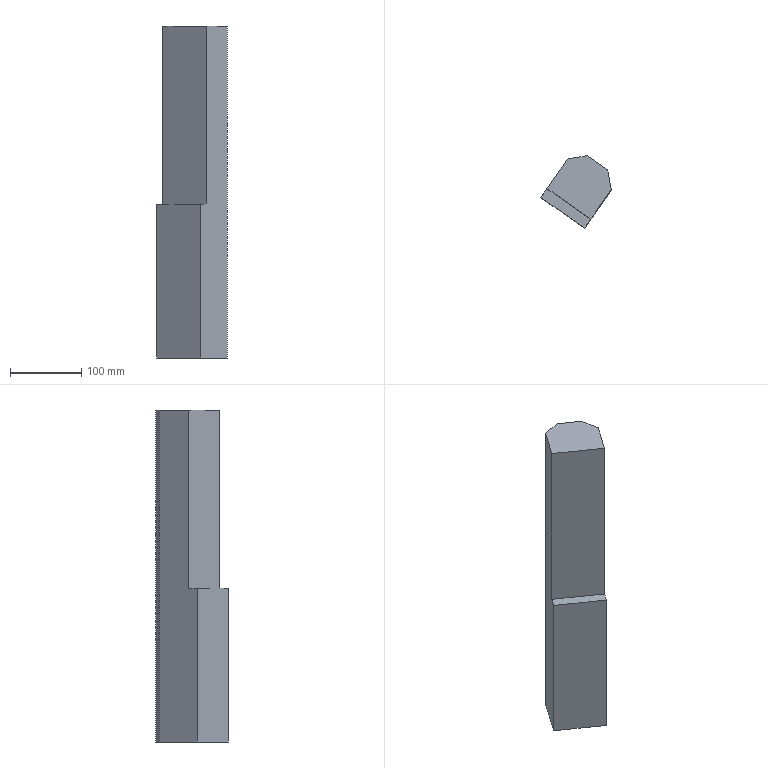Part | NX | features solid 2 | 1 solid | 20 faces | box 98.719 x 101.175 x 465 mm | volume 2453936 mm3 | plane 12 | cylinder 5 | cone 3 | commonest cylinder face diameters 16 x5
STEP:
#1=CARTESIAN_POINT('',(345.382,545.56,-124.062));
#2=VERTEX_POINT('',#1);
#3=CARTESIAN_POINT('',(374.061,586.518,-124.062));
#4=VERTEX_POINT('',#3);
#5=CARTESIAN_POINT('',(345.382,545.56,-124.062));
#6=DIRECTION('',(-0.5736,-0.8192,0.));
#7=VECTOR('',#6,1000.);
#8=LINE('',#5,#7);
#9=EDGE_CURVE('',#2,#4,#8,.F.);
#10=ORIENTED_EDGE('',*,*,#9,.T.);
#11=CARTESIAN_POINT('',(369.15,614.373,-124.062));
#12=VERTEX_POINT('',#11);
#13=CARTESIAN_POINT('',(374.061,586.518,-124.062));
#14=DIRECTION('',(-0.1736,0.9848,0.));
#15=VECTOR('',#14,1000.);
#16=LINE('',#13,#15);
#17=EDGE_CURVE('',#4,#12,#16,.T.);
#18=ORIENTED_EDGE('',*,*,#17,.T.);
#19=CARTESIAN_POINT('',(340.479,634.448,-124.062));
#20=VERTEX_POINT('',#19);
#21=CARTESIAN_POINT('',(324.096,645.919,-124.062));
#22=DIRECTION('',(-0.8192,0.5736,0.));
#23=VECTOR('',#22,1000.);
#24=LINE('',#21,#23);
#25=EDGE_CURVE('',#12,#20,#24,.T.);
#26=ORIENTED_EDGE('',*,*,#25,.T.);
#27=CARTESIAN_POINT('',(312.625,629.536,-124.062));
#28=VERTEX_POINT('',#27);
#29=CARTESIAN_POINT('',(312.625,629.536,-124.062));
#30=DIRECTION('',(-0.9848,-0.1736,0.));
#31=VECTOR('',#30,1000.);
#32=LINE('',#29,#31);
#33=EDGE_CURVE('',#20,#28,#32,.T.);
#34=ORIENTED_EDGE('',*,*,#33,.T.);
#35=CARTESIAN_POINT('',(283.946,588.579,-124.062));
#36=VERTEX_POINT('',#35);
#37=CARTESIAN_POINT('',(283.946,588.579,-124.062));
#38=DIRECTION('',(0.5736,0.8192,0.));
#39=VECTOR('',#38,1000.);
#40=LINE('',#37,#39);
#41=EDGE_CURVE('',#36,#28,#40,.T.);
#42=ORIENTED_EDGE('',*,*,#41,.F.);
#43=CARTESIAN_POINT('',(283.946,588.579,-124.062));
#44=DIRECTION('',(0.8192,-0.5736,0.));
#45=VECTOR('',#44,1000.);
#46=LINE('',#43,#45);
#47=EDGE_CURVE('',#36,#2,#46,.T.);
#48=ORIENTED_EDGE('',*,*,#47,.T.);
#49=EDGE_LOOP('',(#10,#18,#26,#34,#42,#48));
#50=FACE_BOUND('',#49,.T.);
#51=CARTESIAN_POINT('',(283.946,588.579,-124.062));
#52=DIRECTION('',(0.,0.,-1.));
#53=DIRECTION('',(0.5736,0.8192,0.));
#54=AXIS2_PLACEMENT_3D('',#51,#52,#53);
#55=PLANE('',#54);
#56=ADVANCED_FACE('',(#50),#55,.F.);
#57=CARTESIAN_POINT('',(345.382,545.56,-374.062));
#58=VERTEX_POINT('',#57);
#59=CARTESIAN_POINT('',(345.382,545.56,-401.082));
#60=DIRECTION('',(0.,0.,-1.));
#61=VECTOR('',#60,1000.);
#62=LINE('',#59,#61);
#63=EDGE_CURVE('',#2,#58,#62,.T.);
#64=ORIENTED_EDGE('',*,*,#63,.F.);
#65=ORIENTED_EDGE('',*,*,#47,.F.);
#66=CARTESIAN_POINT('',(283.946,588.579,-374.062));
#67=VERTEX_POINT('',#66);
#68=CARTESIAN_POINT('',(283.946,588.579,-401.082));
#69=DIRECTION('',(0.,0.,-1.));
#70=VECTOR('',#69,1000.);
#71=LINE('',#68,#70);
#72=EDGE_CURVE('',#36,#67,#71,.T.);
#73=ORIENTED_EDGE('',*,*,#72,.T.);
#74=CARTESIAN_POINT('',(337.191,551.296,-374.062));
#75=DIRECTION('',(-0.8192,0.5736,0.));
#76=VECTOR('',#75,1000.);
#77=LINE('',#74,#76);
#78=EDGE_CURVE('',#58,#67,#77,.T.);
#79=ORIENTED_EDGE('',*,*,#78,.F.);
#80=EDGE_LOOP('',(#64,#65,#73,#79));
#81=FACE_BOUND('',#80,.T.);
#82=CARTESIAN_POINT('',(283.946,588.579,-401.082));
#83=DIRECTION('',(0.5736,0.8192,0.));
#84=DIRECTION('',(0.8192,-0.5736,0.));
#85=AXIS2_PLACEMENT_3D('',#82,#83,#84);
#86=PLANE('',#85);
#87=ADVANCED_FACE('',(#81),#86,.F.);
#88=CARTESIAN_POINT('',(336.779,533.273,-374.062));
#89=VERTEX_POINT('',#88);
#90=CARTESIAN_POINT('',(336.779,533.273,-589.062));
#91=VERTEX_POINT('',#90);
#92=CARTESIAN_POINT('',(336.779,533.273,-461.082));
#93=DIRECTION('',(0.,0.,1.));
#94=VECTOR('',#93,1000.);
#95=LINE('',#92,#94);
#96=EDGE_CURVE('',#89,#91,#95,.F.);
#97=ORIENTED_EDGE('',*,*,#96,.F.);
#98=CARTESIAN_POINT('',(275.342,576.291,-374.062));
#99=VERTEX_POINT('',#98);
#100=CARTESIAN_POINT('',(328.587,539.009,-374.062));
#101=DIRECTION('',(-0.8192,0.5736,0.));
#102=VECTOR('',#101,1000.);
#103=LINE('',#100,#102);
#104=EDGE_CURVE('',#89,#99,#103,.T.);
#105=ORIENTED_EDGE('',*,*,#104,.T.);
#106=CARTESIAN_POINT('',(275.342,576.291,-589.062));
#107=VERTEX_POINT('',#106);
#108=CARTESIAN_POINT('',(275.342,576.291,-401.082));
#109=DIRECTION('',(0.,0.,-1.));
#110=VECTOR('',#109,1000.);
#111=LINE('',#108,#110);
#112=EDGE_CURVE('',#99,#107,#111,.T.);
#113=ORIENTED_EDGE('',*,*,#112,.T.);
#114=CARTESIAN_POINT('',(275.26,576.349,-589.062));
#115=DIRECTION('',(0.8192,-0.5736,0.));
#116=VECTOR('',#115,1000.);
#117=LINE('',#114,#116);
#118=EDGE_CURVE('',#91,#107,#117,.F.);
#119=ORIENTED_EDGE('',*,*,#118,.F.);
#120=EDGE_LOOP('',(#97,#105,#113,#119));
#121=FACE_BOUND('',#120,.T.);
#122=CARTESIAN_POINT('',(328.587,539.009,-461.082));
#123=DIRECTION('',(-0.5736,-0.8192,0.));
#124=DIRECTION('',(-0.8192,0.5736,0.));
#125=AXIS2_PLACEMENT_3D('',#122,#123,#124);
#126=PLANE('',#125);
#127=ADVANCED_FACE('',(#121),#126,.T.);
#128=CARTESIAN_POINT('',(341.074,585.702,-589.062));
#129=VERTEX_POINT('',#128);
#130=CARTESIAN_POINT('',(349.074,585.702,-589.062));
#131=DIRECTION('',(0.,0.,-1.));
#132=DIRECTION('',(-1.,0.,0.));
#133=AXIS2_PLACEMENT_3D('',#130,#131,#132);
#134=CIRCLE('',#133,8.);
#135=EDGE_CURVE('',#129,#129,#134,.F.);
#136=ORIENTED_EDGE('',*,*,#135,.T.);
#137=EDGE_LOOP('',(#136));
#138=FACE_BOUND('',#137,.T.);
#139=CARTESIAN_POINT('',(309.536,601.682,-589.062));
#140=VERTEX_POINT('',#139);
#141=CARTESIAN_POINT('',(317.536,601.682,-589.062));
#142=DIRECTION('',(0.,0.,-1.));
#143=DIRECTION('',(-1.,0.,0.));
#144=AXIS2_PLACEMENT_3D('',#141,#142,#143);
#145=CIRCLE('',#144,8.);
#146=EDGE_CURVE('',#140,#140,#145,.F.);
#147=ORIENTED_EDGE('',*,*,#146,.T.);
#148=EDGE_LOOP('',(#147));
#149=FACE_BOUND('',#148,.T.);
#150=CARTESIAN_POINT('',(349.295,609.461,-589.062));
#151=VERTEX_POINT('',#150);
#152=CARTESIAN_POINT('',(341.295,609.461,-589.062));
#153=DIRECTION('',(0.,0.,1.));
#154=DIRECTION('',(1.,0.,0.));
#155=AXIS2_PLACEMENT_3D('',#152,#153,#154);
#156=CIRCLE('',#155,8.);
#157=EDGE_CURVE('',#151,#151,#156,.T.);
#158=ORIENTED_EDGE('',*,*,#157,.T.);
#159=EDGE_LOOP('',(#158));
#160=FACE_BOUND('',#159,.T.);
#161=CARTESIAN_POINT('',(311.197,581.203,-589.062));
#162=VERTEX_POINT('',#161);
#163=CARTESIAN_POINT('',(303.197,581.203,-589.062));
#164=DIRECTION('',(0.,0.,1.));
#165=DIRECTION('',(1.,0.,0.));
#166=AXIS2_PLACEMENT_3D('',#163,#164,#165);
#167=CIRCLE('',#166,8.);
#168=EDGE_CURVE('',#162,#162,#167,.T.);
#169=ORIENTED_EDGE('',*,*,#168,.T.);
#170=EDGE_LOOP('',(#169));
#171=FACE_BOUND('',#170,.T.);
#172=CARTESIAN_POINT('',(339.867,561.128,-589.062));
#173=VERTEX_POINT('',#172);
#174=CARTESIAN_POINT('',(331.867,561.128,-589.062));
#175=DIRECTION('',(0.,0.,1.));
#176=DIRECTION('',(1.,0.,0.));
#177=AXIS2_PLACEMENT_3D('',#174,#175,#176);
#178=CIRCLE('',#177,8.);
#179=EDGE_CURVE('',#173,#173,#178,.T.);
#180=ORIENTED_EDGE('',*,*,#179,.T.);
#181=EDGE_LOOP('',(#180));
#182=FACE_BOUND('',#181,.T.);
#183=CARTESIAN_POINT('',(369.15,614.373,-589.062));
#184=VERTEX_POINT('',#183);
#185=CARTESIAN_POINT('',(340.479,634.448,-589.062));
#186=VERTEX_POINT('',#185);
#187=CARTESIAN_POINT('',(-187.66,1004.255,-589.062));
#188=DIRECTION('',(0.8192,-0.5736,0.));
#189=VECTOR('',#188,1000.);
#190=LINE('',#187,#189);
#191=EDGE_CURVE('',#184,#186,#190,.F.);
#192=ORIENTED_EDGE('',*,*,#191,.F.);
#193=CARTESIAN_POINT('',(374.061,586.518,-589.062));
#194=VERTEX_POINT('',#193);
#195=CARTESIAN_POINT('',(374.061,586.518,-589.062));
#196=DIRECTION('',(-0.1736,0.9848,0.));
#197=VECTOR('',#196,1000.);
#198=LINE('',#195,#197);
#199=EDGE_CURVE('',#184,#194,#198,.F.);
#200=ORIENTED_EDGE('',*,*,#199,.T.);
#201=CARTESIAN_POINT('',(256.478,418.592,-589.062));
#202=DIRECTION('',(0.5736,0.8192,0.));
#203=VECTOR('',#202,1000.);
#204=LINE('',#201,#203);
#205=EDGE_CURVE('',#91,#194,#204,.T.);
#206=ORIENTED_EDGE('',*,*,#205,.F.);
#207=ORIENTED_EDGE('',*,*,#118,.T.);
#208=CARTESIAN_POINT('',(312.625,629.536,-589.062));
#209=VERTEX_POINT('',#208);
#210=CARTESIAN_POINT('',(344.171,674.59,-589.062));
#211=DIRECTION('',(-0.5736,-0.8192,0.));
#212=VECTOR('',#211,1000.);
#213=LINE('',#210,#212);
#214=EDGE_CURVE('',#107,#209,#213,.F.);
#215=ORIENTED_EDGE('',*,*,#214,.T.);
#216=CARTESIAN_POINT('',(312.625,629.536,-589.062));
#217=DIRECTION('',(-0.9848,-0.1736,0.));
#218=VECTOR('',#217,1000.);
#219=LINE('',#216,#218);
#220=EDGE_CURVE('',#209,#186,#219,.F.);
#221=ORIENTED_EDGE('',*,*,#220,.T.);
#222=EDGE_LOOP('',(#192,#200,#206,#207,#215,#221));
#223=FACE_BOUND('',#222,.T.);
#224=CARTESIAN_POINT('',(344.089,674.647,-589.062));
#225=DIRECTION('',(0.,0.,-1.));
#226=DIRECTION('',(-0.5736,-0.8192,0.));
#227=AXIS2_PLACEMENT_3D('',#224,#225,#226);
#228=PLANE('',#227);
#229=ADVANCED_FACE('',(#138,#149,#160,#171,#182,#223),#228,.T.);
#230=ORIENTED_EDGE('',*,*,#41,.T.);
#231=CARTESIAN_POINT('',(312.625,629.536,-589.062));
#232=DIRECTION('',(0.,0.,-1.));
#233=VECTOR('',#232,1000.);
#234=LINE('',#231,#233);
#235=EDGE_CURVE('',#28,#209,#234,.T.);
#236=ORIENTED_EDGE('',*,*,#235,.T.);
#237=ORIENTED_EDGE('',*,*,#214,.F.);
#238=ORIENTED_EDGE('',*,*,#112,.F.);
#239=CARTESIAN_POINT('',(283.946,588.579,-374.062));
#240=DIRECTION('',(0.5736,0.8192,0.));
#241=VECTOR('',#240,1000.);
#242=LINE('',#239,#241);
#243=EDGE_CURVE('',#99,#67,#242,.T.);
#244=ORIENTED_EDGE('',*,*,#243,.T.);
#245=ORIENTED_EDGE('',*,*,#72,.F.);
#246=EDGE_LOOP('',(#230,#236,#237,#238,#244,#245));
#247=FACE_BOUND('',#246,.T.);
#248=CARTESIAN_POINT('',(283.946,588.579,-151.082));
#249=DIRECTION('',(-0.8192,0.5736,0.));
#250=DIRECTION('',(0.5736,0.8192,0.));
#251=AXIS2_PLACEMENT_3D('',#248,#249,#250);
#252=PLANE('',#251);
#253=ADVANCED_FACE('',(#247),#252,.T.);
#254=ORIENTED_EDGE('',*,*,#25,.F.);
#255=CARTESIAN_POINT('',(369.15,614.373,-192.696));
#256=DIRECTION('',(0.,0.,-1.));
#257=VECTOR('',#256,1000.);
#258=LINE('',#255,#257);
#259=EDGE_CURVE('',#12,#184,#258,.T.);
#260=ORIENTED_EDGE('',*,*,#259,.T.);
#261=ORIENTED_EDGE('',*,*,#191,.T.);
#262=CARTESIAN_POINT('',(340.479,634.448,-124.062));
#263=DIRECTION('',(0.,0.,1.));
#264=VECTOR('',#263,1000.);
#265=LINE('',#262,#264);
#266=EDGE_CURVE('',#186,#20,#265,.T.);
#267=ORIENTED_EDGE('',*,*,#266,.T.);
#268=EDGE_LOOP('',(#254,#260,#261,#267));
#269=FACE_BOUND('',#268,.T.);
#270=CARTESIAN_POINT('',(-187.66,1004.255,-192.696));
#271=DIRECTION('',(-0.5736,-0.8192,0.));
#272=DIRECTION('',(-0.8192,0.5736,0.));
#273=AXIS2_PLACEMENT_3D('',#270,#271,#272);
#274=PLANE('',#273);
#275=ADVANCED_FACE('',(#269),#274,.F.);
#276=CARTESIAN_POINT('',(345.382,545.56,-374.062));
#277=DIRECTION('',(0.5736,0.8192,0.));
#278=VECTOR('',#277,1000.);
#279=LINE('',#276,#278);
#280=EDGE_CURVE('',#89,#58,#279,.T.);
#281=ORIENTED_EDGE('',*,*,#280,.T.);
#282=ORIENTED_EDGE('',*,*,#78,.T.);
#283=ORIENTED_EDGE('',*,*,#243,.F.);
#284=ORIENTED_EDGE('',*,*,#104,.F.);
#285=EDGE_LOOP('',(#281,#282,#283,#284));
#286=FACE_BOUND('',#285,.T.);
#287=CARTESIAN_POINT('',(337.191,551.296,-374.062));
#288=DIRECTION('',(0.,0.,1.));
#289=DIRECTION('',(-0.5736,-0.8192,0.));
#290=AXIS2_PLACEMENT_3D('',#287,#288,#289);
#291=PLANE('',#290);
#292=ADVANCED_FACE('',(#286),#291,.T.);
#293=ORIENTED_EDGE('',*,*,#205,.T.);
#294=CARTESIAN_POINT('',(374.061,586.518,-400.));
#295=DIRECTION('',(0.,0.,-1.));
#296=VECTOR('',#295,1000.);
#297=LINE('',#294,#296);
#298=EDGE_CURVE('',#194,#4,#297,.F.);
#299=ORIENTED_EDGE('',*,*,#298,.T.);
#300=ORIENTED_EDGE('',*,*,#9,.F.);
#301=ORIENTED_EDGE('',*,*,#63,.T.);
#302=ORIENTED_EDGE('',*,*,#280,.F.);
#303=ORIENTED_EDGE('',*,*,#96,.T.);
#304=EDGE_LOOP('',(#293,#299,#300,#301,#302,#303));
#305=FACE_BOUND('',#304,.T.);
#306=CARTESIAN_POINT('',(256.478,418.592,-400.));
#307=DIRECTION('',(0.8192,-0.5736,0.));
#308=DIRECTION('',(0.,0.,1.));
#309=AXIS2_PLACEMENT_3D('',#306,#307,#308);
#310=PLANE('',#309);
#311=ADVANCED_FACE('',(#305),#310,.T.);
#312=ORIENTED_EDGE('',*,*,#33,.F.);
#313=ORIENTED_EDGE('',*,*,#266,.F.);
#314=ORIENTED_EDGE('',*,*,#220,.F.);
#315=ORIENTED_EDGE('',*,*,#235,.F.);
#316=EDGE_LOOP('',(#312,#313,#314,#315));
#317=FACE_BOUND('',#316,.T.);
#318=CARTESIAN_POINT('',(312.625,629.536,-151.082));
#319=DIRECTION('',(-0.1736,0.9848,0.));
#320=DIRECTION('',(-0.9848,-0.1736,0.));
#321=AXIS2_PLACEMENT_3D('',#318,#319,#320);
#322=PLANE('',#321);
#323=ADVANCED_FACE('',(#317),#322,.T.);
#324=ORIENTED_EDGE('',*,*,#199,.F.);
#325=ORIENTED_EDGE('',*,*,#259,.F.);
#326=ORIENTED_EDGE('',*,*,#17,.F.);
#327=ORIENTED_EDGE('',*,*,#298,.F.);
#328=EDGE_LOOP('',(#324,#325,#326,#327));
#329=FACE_BOUND('',#328,.T.);
#330=CARTESIAN_POINT('',(374.061,586.518,-400.));
#331=DIRECTION('',(0.9848,0.1736,0.));
#332=DIRECTION('',(-0.1736,0.9848,0.));
#333=AXIS2_PLACEMENT_3D('',#330,#331,#332);
#334=PLANE('',#333);
#335=ADVANCED_FACE('',(#329),#334,.T.);
#336=CARTESIAN_POINT('',(339.867,561.128,-539.062));
#337=VERTEX_POINT('',#336);
#338=CARTESIAN_POINT('',(331.867,561.128,-539.062));
#339=DIRECTION('',(0.,0.,1.));
#340=DIRECTION('',(1.,0.,0.));
#341=AXIS2_PLACEMENT_3D('',#338,#339,#340);
#342=CIRCLE('',#341,8.);
#343=EDGE_CURVE('',#337,#337,#342,.T.);
#344=ORIENTED_EDGE('',*,*,#343,.F.);
#345=EDGE_LOOP('',(#344));
#346=FACE_BOUND('',#345,.T.);
#347=CARTESIAN_POINT('',(331.867,561.128,-534.256));
#348=VERTEX_POINT('',#347);
#349=VERTEX_LOOP('',#348);
#350=FACE_BOUND('',#349,.T.);
#351=CARTESIAN_POINT('',(331.867,561.128,-539.062));
#352=DIRECTION('',(0.,0.,-1.));
#353=DIRECTION('',(-1.,0.,0.));
#354=AXIS2_PLACEMENT_3D('',#351,#352,#353);
#355=CONICAL_SURFACE('',#354,8.,1.03);
#356=ADVANCED_FACE('',(#346,#350),#355,.F.);
#357=ORIENTED_EDGE('',*,*,#343,.T.);
#358=EDGE_LOOP('',(#357));
#359=FACE_BOUND('',#358,.T.);
#360=ORIENTED_EDGE('',*,*,#179,.F.);
#361=EDGE_LOOP('',(#360));
#362=FACE_BOUND('',#361,.T.);
#363=CARTESIAN_POINT('',(331.867,561.128,-589.062));
#364=DIRECTION('',(0.,0.,1.));
#365=DIRECTION('',(1.,0.,0.));
#366=AXIS2_PLACEMENT_3D('',#363,#364,#365);
#367=CYLINDRICAL_SURFACE('',#366,8.);
#368=ADVANCED_FACE('',(#359,#362),#367,.F.);
#369=CARTESIAN_POINT('',(311.197,581.203,-539.062));
#370=VERTEX_POINT('',#369);
#371=CARTESIAN_POINT('',(303.197,581.203,-539.062));
#372=DIRECTION('',(0.,0.,1.));
#373=DIRECTION('',(1.,0.,0.));
#374=AXIS2_PLACEMENT_3D('',#371,#372,#373);
#375=CIRCLE('',#374,8.);
#376=EDGE_CURVE('',#370,#370,#375,.T.);
#377=ORIENTED_EDGE('',*,*,#376,.F.);
#378=EDGE_LOOP('',(#377));
#379=FACE_BOUND('',#378,.T.);
#380=CARTESIAN_POINT('',(303.197,581.203,-534.256));
#381=VERTEX_POINT('',#380);
#382=VERTEX_LOOP('',#381);
#383=FACE_BOUND('',#382,.T.);
#384=CARTESIAN_POINT('',(303.197,581.203,-539.062));
#385=DIRECTION('',(0.,0.,-1.));
#386=DIRECTION('',(-1.,0.,0.));
#387=AXIS2_PLACEMENT_3D('',#384,#385,#386);
#388=CONICAL_SURFACE('',#387,8.,1.03);
#389=ADVANCED_FACE('',(#379,#383),#388,.F.);
#390=ORIENTED_EDGE('',*,*,#376,.T.);
#391=EDGE_LOOP('',(#390));
#392=FACE_BOUND('',#391,.T.);
#393=ORIENTED_EDGE('',*,*,#168,.F.);
#394=EDGE_LOOP('',(#393));
#395=FACE_BOUND('',#394,.T.);
#396=CARTESIAN_POINT('',(303.197,581.203,-589.062));
#397=DIRECTION('',(0.,0.,1.));
#398=DIRECTION('',(1.,0.,0.));
#399=AXIS2_PLACEMENT_3D('',#396,#397,#398);
#400=CYLINDRICAL_SURFACE('',#399,8.);
#401=ADVANCED_FACE('',(#392,#395),#400,.F.);
#402=CARTESIAN_POINT('',(349.295,609.461,-539.062));
#403=VERTEX_POINT('',#402);
#404=CARTESIAN_POINT('',(341.295,609.461,-539.062));
#405=DIRECTION('',(0.,0.,1.));
#406=DIRECTION('',(1.,0.,0.));
#407=AXIS2_PLACEMENT_3D('',#404,#405,#406);
#408=CIRCLE('',#407,8.);
#409=EDGE_CURVE('',#403,#403,#408,.T.);
#410=ORIENTED_EDGE('',*,*,#409,.F.);
#411=EDGE_LOOP('',(#410));
#412=FACE_BOUND('',#411,.T.);
#413=CARTESIAN_POINT('',(341.295,609.461,-534.256));
#414=VERTEX_POINT('',#413);
#415=VERTEX_LOOP('',#414);
#416=FACE_BOUND('',#415,.T.);
#417=CARTESIAN_POINT('',(341.295,609.461,-539.062));
#418=DIRECTION('',(0.,0.,-1.));
#419=DIRECTION('',(-1.,0.,0.));
#420=AXIS2_PLACEMENT_3D('',#417,#418,#419);
#421=CONICAL_SURFACE('',#420,8.,1.03);
#422=ADVANCED_FACE('',(#412,#416),#421,.F.);
#423=ORIENTED_EDGE('',*,*,#409,.T.);
#424=EDGE_LOOP('',(#423));
#425=FACE_BOUND('',#424,.T.);
#426=ORIENTED_EDGE('',*,*,#157,.F.);
#427=EDGE_LOOP('',(#426));
#428=FACE_BOUND('',#427,.T.);
#429=CARTESIAN_POINT('',(341.295,609.461,-589.062));
#430=DIRECTION('',(0.,0.,1.));
#431=DIRECTION('',(1.,0.,0.));
#432=AXIS2_PLACEMENT_3D('',#429,#430,#431);
#433=CYLINDRICAL_SURFACE('',#432,8.);
#434=ADVANCED_FACE('',(#425,#428),#433,.F.);
#435=CARTESIAN_POINT('',(325.536,601.682,-559.062));
#436=VERTEX_POINT('',#435);
#437=CARTESIAN_POINT('',(317.536,601.682,-559.062));
#438=DIRECTION('',(0.,0.,1.));
#439=DIRECTION('',(1.,0.,0.));
#440=AXIS2_PLACEMENT_3D('',#437,#438,#439);
#441=CIRCLE('',#440,8.);
#442=EDGE_CURVE('',#436,#436,#441,.T.);
#443=ORIENTED_EDGE('',*,*,#442,.T.);
#444=EDGE_LOOP('',(#443));
#445=FACE_BOUND('',#444,.T.);
#446=ORIENTED_EDGE('',*,*,#146,.F.);
#447=EDGE_LOOP('',(#446));
#448=FACE_BOUND('',#447,.T.);
#449=CARTESIAN_POINT('',(317.536,601.682,-689.062));
#450=DIRECTION('',(0.,0.,1.));
#451=DIRECTION('',(1.,0.,0.));
#452=AXIS2_PLACEMENT_3D('',#449,#450,#451);
#453=CYLINDRICAL_SURFACE('',#452,8.);
#454=ADVANCED_FACE('',(#445,#448),#453,.F.);
#455=ORIENTED_EDGE('',*,*,#442,.F.);
#456=EDGE_LOOP('',(#455));
#457=FACE_BOUND('',#456,.T.);
#458=CARTESIAN_POINT('',(317.536,601.682,-559.062));
#459=DIRECTION('',(0.,0.,1.));
#460=DIRECTION('',(1.,0.,0.));
#461=AXIS2_PLACEMENT_3D('',#458,#459,#460);
#462=PLANE('',#461);
#463=ADVANCED_FACE('',(#457),#462,.F.);
#464=CARTESIAN_POINT('',(357.074,585.702,-559.062));
#465=VERTEX_POINT('',#464);
#466=CARTESIAN_POINT('',(349.074,585.702,-559.062));
#467=DIRECTION('',(0.,0.,1.));
#468=DIRECTION('',(1.,0.,0.));
#469=AXIS2_PLACEMENT_3D('',#466,#467,#468);
#470=CIRCLE('',#469,8.);
#471=EDGE_CURVE('',#465,#465,#470,.T.);
#472=ORIENTED_EDGE('',*,*,#471,.T.);
#473=EDGE_LOOP('',(#472));
#474=FACE_BOUND('',#473,.T.);
#475=ORIENTED_EDGE('',*,*,#135,.F.);
#476=EDGE_LOOP('',(#475));
#477=FACE_BOUND('',#476,.T.);
#478=CARTESIAN_POINT('',(349.074,585.702,-689.062));
#479=DIRECTION('',(0.,0.,1.));
#480=DIRECTION('',(1.,0.,0.));
#481=AXIS2_PLACEMENT_3D('',#478,#479,#480);
#482=CYLINDRICAL_SURFACE('',#481,8.);
#483=ADVANCED_FACE('',(#474,#477),#482,.F.);
#484=ORIENTED_EDGE('',*,*,#471,.F.);
#485=EDGE_LOOP('',(#484));
#486=FACE_BOUND('',#485,.T.);
#487=CARTESIAN_POINT('',(349.074,585.702,-559.062));
#488=DIRECTION('',(0.,0.,1.));
#489=DIRECTION('',(1.,0.,0.));
#490=AXIS2_PLACEMENT_3D('',#487,#488,#489);
#491=PLANE('',#490);
#492=ADVANCED_FACE('',(#486),#491,.F.);
#493=CLOSED_SHELL('',(#56,#87,#127,#229,#253,#275,#292,#311,#323,#335,#356,#368,#389,#401,#422,#434,#454,#463,#483,#492));
#494=MANIFOLD_SOLID_BREP('',#493);
#495=(LENGTH_UNIT()NAMED_UNIT(*)SI_UNIT(.MILLI.,.METRE.));
#496=UNCERTAINTY_MEASURE_WITH_UNIT(LENGTH_MEASURE(0.00001),#495,'','');
#497=(NAMED_UNIT(*)PLANE_ANGLE_UNIT()SI_UNIT($,.RADIAN.));
#498=(NAMED_UNIT(*)SI_UNIT($,.STERADIAN.)SOLID_ANGLE_UNIT());
#499=(GEOMETRIC_REPRESENTATION_CONTEXT(3)GLOBAL_UNCERTAINTY_ASSIGNED_CONTEXT((#496))GLOBAL_UNIT_ASSIGNED_CONTEXT((#495,#497,#498))REPRESENTATION_CONTEXT('',''));
#500=ADVANCED_BREP_SHAPE_REPRESENTATION('',(#494),#499);